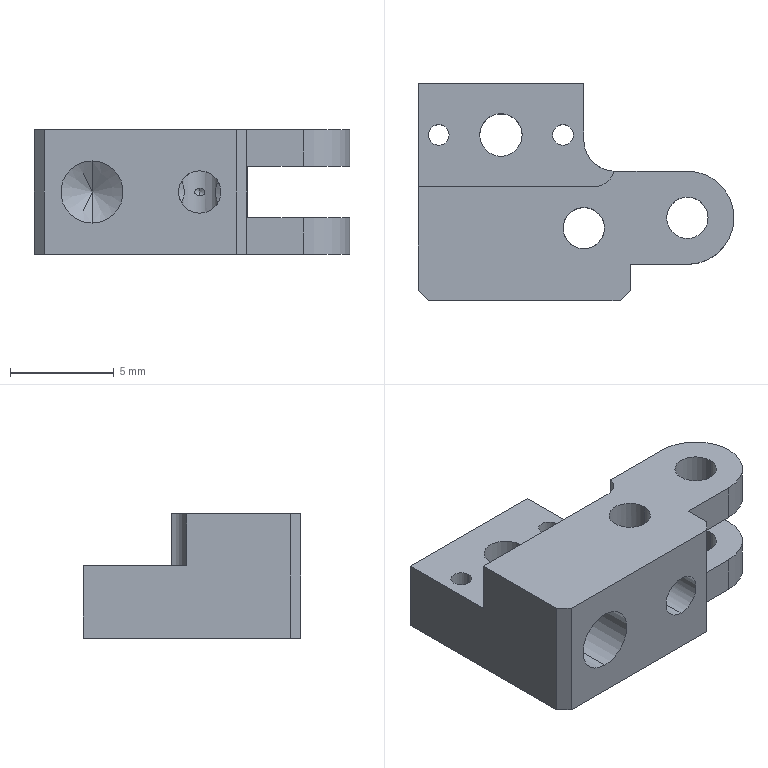Part | SolidWorks | features HoleWzd 5, ICE 5, Fillet 2, Chamfer 1, Extrusion 1 | 1 solid | 45 faces | box 15.25 x 10.5 x 6 mm | volume 471.852 mm3 | cylinder 23 | plane 16 | cone 6 | commonest cylinder face diameters 2 x8 1 x4 2.05 x4 4.5 x4 3 x3